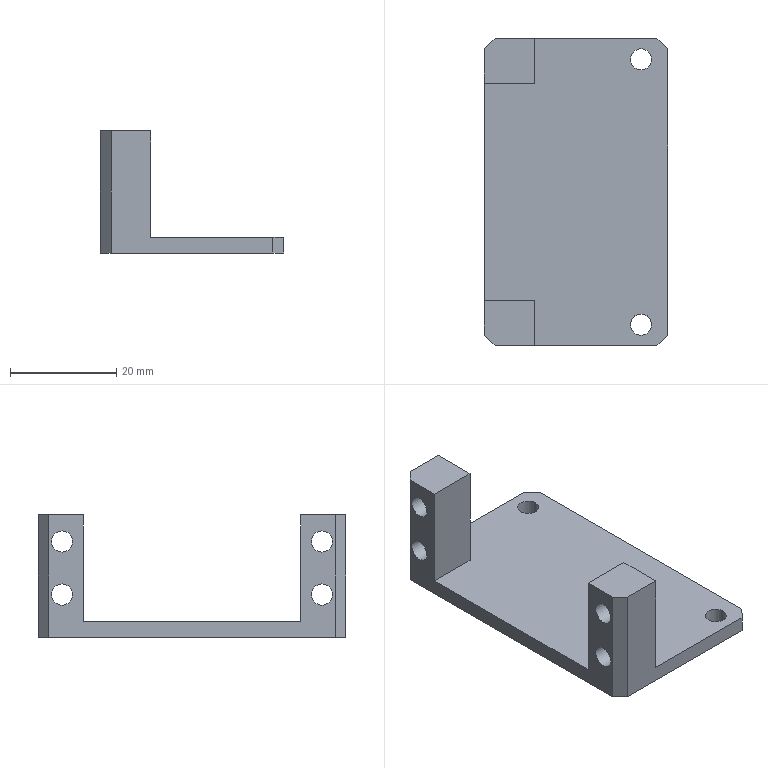Part | STEP file | Servo fixing bracket-Y-middle | 1 solid | 22 faces | box 34.5 x 58 x 23 mm | volume 8576 mm3 | plane 16 | cylinder 6 | commonest cylinder face diameters 4 x6